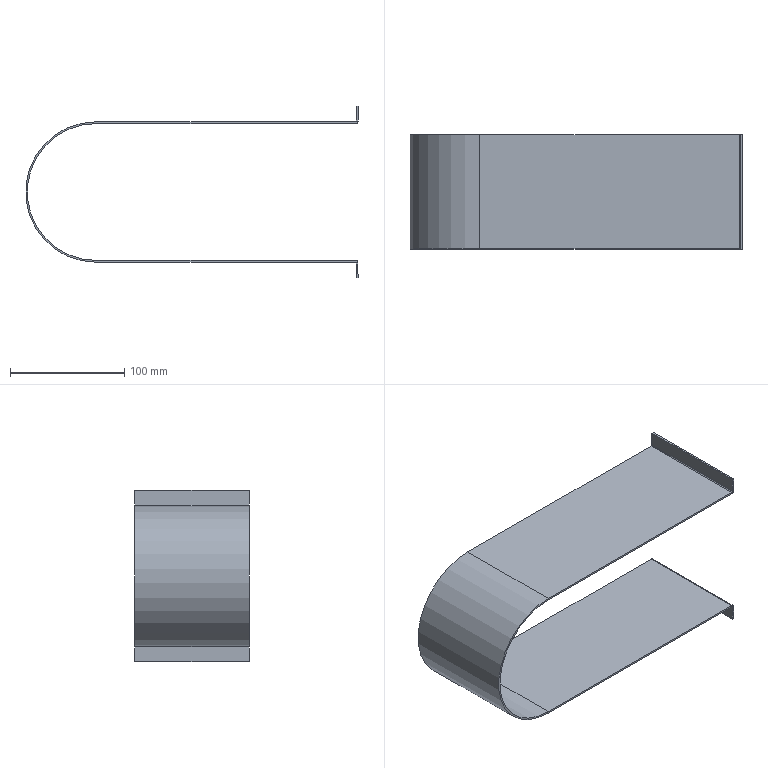Part | SolidWorks | features BaseBody 1 | 1 solid | 18 faces | box 291.5 x 100 x 150 mm | volume 101486 mm3 | plane 12 | cylinder 6 | commonest cylinder face diameters 1.473 x2 4.473 x2 120 x1 123 x1
STEP:
#1=CARTESIAN_POINT('',(-115.,100.,60.));
#2=VERTEX_POINT('',#1);
#3=CARTESIAN_POINT('',(112.763,100.,60.));
#4=VERTEX_POINT('',#3);
#5=CARTESIAN_POINT('',(-115.,100.,60.));
#6=DIRECTION('',(1.,0.,0.));
#7=VECTOR('',#6,1000.);
#8=LINE('',#5,#7);
#9=EDGE_CURVE('',#2,#4,#8,.T.);
#10=ORIENTED_EDGE('',*,*,#9,.T.);
#11=CARTESIAN_POINT('',(112.763,0.,60.));
#12=VERTEX_POINT('',#11);
#13=CARTESIAN_POINT('',(112.763,100.,60.));
#14=DIRECTION('',(0.,-1.,0.));
#15=VECTOR('',#14,1000.);
#16=LINE('',#13,#15);
#17=EDGE_CURVE('',#4,#12,#16,.T.);
#18=ORIENTED_EDGE('',*,*,#17,.T.);
#19=CARTESIAN_POINT('',(-115.,0.,60.));
#20=VERTEX_POINT('',#19);
#21=CARTESIAN_POINT('',(-115.,0.,60.));
#22=DIRECTION('',(-1.,0.,0.));
#23=VECTOR('',#22,1000.);
#24=LINE('',#21,#23);
#25=EDGE_CURVE('',#12,#20,#24,.T.);
#26=ORIENTED_EDGE('',*,*,#25,.T.);
#27=CARTESIAN_POINT('',(-115.,100.,60.));
#28=DIRECTION('',(0.,1.,0.));
#29=VECTOR('',#28,1000.);
#30=LINE('',#27,#29);
#31=EDGE_CURVE('',#20,#2,#30,.T.);
#32=ORIENTED_EDGE('',*,*,#31,.T.);
#33=EDGE_LOOP('',(#10,#18,#26,#32));
#34=FACE_OUTER_BOUND('',#33,.T.);
#35=CARTESIAN_POINT('',(-115.,100.,60.));
#36=DIRECTION('',(0.,0.,-1.));
#37=DIRECTION('',(-1.,0.,0.));
#38=AXIS2_PLACEMENT_3D('',#35,#36,#37);
#39=PLANE('',#38);
#40=ADVANCED_FACE('',(#34),#39,.T.);
#41=CARTESIAN_POINT('',(115.,100.,62.237));
#42=VERTEX_POINT('',#41);
#43=CARTESIAN_POINT('',(112.763,100.,62.237));
#44=DIRECTION('',(0.,-1.,0.));
#45=DIRECTION('',(0.,0.,-1.));
#46=AXIS2_PLACEMENT_3D('',#43,#44,#45);
#47=CIRCLE('',#46,2.237);
#48=EDGE_CURVE('',#4,#42,#47,.T.);
#49=ORIENTED_EDGE('',*,*,#48,.T.);
#50=CARTESIAN_POINT('',(115.,0.,62.237));
#51=VERTEX_POINT('',#50);
#52=CARTESIAN_POINT('',(115.,100.,62.237));
#53=DIRECTION('',(0.,-1.,0.));
#54=VECTOR('',#53,1000.);
#55=LINE('',#52,#54);
#56=EDGE_CURVE('',#42,#51,#55,.T.);
#57=ORIENTED_EDGE('',*,*,#56,.T.);
#58=CARTESIAN_POINT('',(112.763,0.,62.237));
#59=DIRECTION('',(0.,1.,0.));
#60=DIRECTION('',(0.,0.,-1.));
#61=AXIS2_PLACEMENT_3D('',#58,#59,#60);
#62=CIRCLE('',#61,2.237);
#63=EDGE_CURVE('',#51,#12,#62,.T.);
#64=ORIENTED_EDGE('',*,*,#63,.T.);
#65=ORIENTED_EDGE('',*,*,#17,.F.);
#66=EDGE_LOOP('',(#49,#57,#64,#65));
#67=FACE_OUTER_BOUND('',#66,.T.);
#68=CARTESIAN_POINT('',(112.763,100.,62.237));
#69=DIRECTION('',(0.,-1.,0.));
#70=DIRECTION('',(0.,0.,-1.));
#71=AXIS2_PLACEMENT_3D('',#68,#69,#70);
#72=CYLINDRICAL_SURFACE('',#71,2.237);
#73=ADVANCED_FACE('',(#67),#72,.T.);
#74=CARTESIAN_POINT('',(-115.,100.,61.5));
#75=VERTEX_POINT('',#74);
#76=CARTESIAN_POINT('',(112.763,100.,61.5));
#77=VERTEX_POINT('',#76);
#78=CARTESIAN_POINT('',(-115.,100.,61.5));
#79=DIRECTION('',(1.,0.,0.));
#80=VECTOR('',#79,1000.);
#81=LINE('',#78,#80);
#82=EDGE_CURVE('',#75,#77,#81,.T.);
#83=ORIENTED_EDGE('',*,*,#82,.T.);
#84=CARTESIAN_POINT('',(113.5,100.,62.237));
#85=VERTEX_POINT('',#84);
#86=CARTESIAN_POINT('',(112.763,100.,62.237));
#87=DIRECTION('',(0.,-1.,0.));
#88=DIRECTION('',(0.,0.,-1.));
#89=AXIS2_PLACEMENT_3D('',#86,#87,#88);
#90=CIRCLE('',#89,0.7366);
#91=EDGE_CURVE('',#77,#85,#90,.T.);
#92=ORIENTED_EDGE('',*,*,#91,.T.);
#93=CARTESIAN_POINT('',(113.5,100.,75.));
#94=VERTEX_POINT('',#93);
#95=CARTESIAN_POINT('',(113.5,100.,61.5));
#96=DIRECTION('',(0.,0.,1.));
#97=VECTOR('',#96,1000.);
#98=LINE('',#95,#97);
#99=EDGE_CURVE('',#85,#94,#98,.T.);
#100=ORIENTED_EDGE('',*,*,#99,.T.);
#101=CARTESIAN_POINT('',(115.,100.,75.));
#102=VERTEX_POINT('',#101);
#103=CARTESIAN_POINT('',(115.,100.,75.));
#104=DIRECTION('',(-1.,0.,0.));
#105=VECTOR('',#104,1000.);
#106=LINE('',#103,#105);
#107=EDGE_CURVE('',#102,#94,#106,.T.);
#108=ORIENTED_EDGE('',*,*,#107,.F.);
#109=CARTESIAN_POINT('',(115.,100.,60.));
#110=DIRECTION('',(0.,0.,1.));
#111=VECTOR('',#110,1000.);
#112=LINE('',#109,#111);
#113=EDGE_CURVE('',#42,#102,#112,.T.);
#114=ORIENTED_EDGE('',*,*,#113,.F.);
#115=ORIENTED_EDGE('',*,*,#48,.F.);
#116=ORIENTED_EDGE('',*,*,#9,.F.);
#117=CARTESIAN_POINT('',(-115.,100.,-60.));
#118=VERTEX_POINT('',#117);
#119=CARTESIAN_POINT('',(-115.,100.,0.));
#120=DIRECTION('',(0.,-1.,0.));
#121=DIRECTION('',(0.,0.,-1.));
#122=AXIS2_PLACEMENT_3D('',#119,#120,#121);
#123=CIRCLE('',#122,60.);
#124=EDGE_CURVE('',#2,#118,#123,.T.);
#125=ORIENTED_EDGE('',*,*,#124,.T.);
#126=CARTESIAN_POINT('',(112.763,100.,-60.));
#127=VERTEX_POINT('',#126);
#128=CARTESIAN_POINT('',(-115.,100.,-60.));
#129=DIRECTION('',(-1.,0.,0.));
#130=VECTOR('',#129,1000.);
#131=LINE('',#128,#130);
#132=EDGE_CURVE('',#127,#118,#131,.T.);
#133=ORIENTED_EDGE('',*,*,#132,.F.);
#134=CARTESIAN_POINT('',(115.,100.,-62.237));
#135=VERTEX_POINT('',#134);
#136=CARTESIAN_POINT('',(112.763,100.,-62.237));
#137=DIRECTION('',(0.,-1.,0.));
#138=DIRECTION('',(0.,0.,-1.));
#139=AXIS2_PLACEMENT_3D('',#136,#137,#138);
#140=CIRCLE('',#139,2.237);
#141=EDGE_CURVE('',#135,#127,#140,.T.);
#142=ORIENTED_EDGE('',*,*,#141,.F.);
#143=CARTESIAN_POINT('',(115.,100.,-75.));
#144=VERTEX_POINT('',#143);
#145=CARTESIAN_POINT('',(115.,100.,-60.));
#146=DIRECTION('',(0.,0.,1.));
#147=VECTOR('',#146,1000.);
#148=LINE('',#145,#147);
#149=EDGE_CURVE('',#144,#135,#148,.T.);
#150=ORIENTED_EDGE('',*,*,#149,.F.);
#151=CARTESIAN_POINT('',(113.5,100.,-75.));
#152=VERTEX_POINT('',#151);
#153=CARTESIAN_POINT('',(112.763,100.,-75.));
#154=DIRECTION('',(-1.,0.,0.));
#155=VECTOR('',#154,1000.);
#156=LINE('',#153,#155);
#157=EDGE_CURVE('',#144,#152,#156,.T.);
#158=ORIENTED_EDGE('',*,*,#157,.T.);
#159=CARTESIAN_POINT('',(113.5,100.,-62.237));
#160=VERTEX_POINT('',#159);
#161=CARTESIAN_POINT('',(113.5,100.,62.237));
#162=DIRECTION('',(0.,0.,1.));
#163=VECTOR('',#162,1000.);
#164=LINE('',#161,#163);
#165=EDGE_CURVE('',#152,#160,#164,.T.);
#166=ORIENTED_EDGE('',*,*,#165,.T.);
#167=CARTESIAN_POINT('',(112.763,100.,-61.5));
#168=VERTEX_POINT('',#167);
#169=CARTESIAN_POINT('',(112.763,100.,-62.237));
#170=DIRECTION('',(0.,-1.,0.));
#171=DIRECTION('',(0.,0.,-1.));
#172=AXIS2_PLACEMENT_3D('',#169,#170,#171);
#173=CIRCLE('',#172,0.7366);
#174=EDGE_CURVE('',#160,#168,#173,.T.);
#175=ORIENTED_EDGE('',*,*,#174,.T.);
#176=CARTESIAN_POINT('',(-115.,100.,-61.5));
#177=VERTEX_POINT('',#176);
#178=CARTESIAN_POINT('',(113.5,100.,-61.5));
#179=DIRECTION('',(-1.,0.,0.));
#180=VECTOR('',#179,1000.);
#181=LINE('',#178,#180);
#182=EDGE_CURVE('',#168,#177,#181,.T.);
#183=ORIENTED_EDGE('',*,*,#182,.T.);
#184=CARTESIAN_POINT('',(-115.,100.,0.));
#185=DIRECTION('',(0.,1.,0.));
#186=DIRECTION('',(0.,0.,-1.));
#187=AXIS2_PLACEMENT_3D('',#184,#185,#186);
#188=CIRCLE('',#187,61.5);
#189=EDGE_CURVE('',#177,#75,#188,.T.);
#190=ORIENTED_EDGE('',*,*,#189,.T.);
#191=EDGE_LOOP('',(#83,#92,#100,#108,#114,#115,#116,#125,#133,#142,#150,#158,#166,#175,#183,#190));
#192=FACE_OUTER_BOUND('',#191,.T.);
#193=CARTESIAN_POINT('',(-115.,100.,-61.5));
#194=DIRECTION('',(0.,1.,0.));
#195=DIRECTION('',(0.,0.,1.));
#196=AXIS2_PLACEMENT_3D('',#193,#194,#195);
#197=PLANE('',#196);
#198=ADVANCED_FACE('',(#192),#197,.T.);
#199=CARTESIAN_POINT('',(-115.,0.,-60.));
#200=VERTEX_POINT('',#199);
#201=CARTESIAN_POINT('',(-115.,100.,-60.));
#202=DIRECTION('',(0.,-1.,0.));
#203=VECTOR('',#202,1000.);
#204=LINE('',#201,#203);
#205=EDGE_CURVE('',#118,#200,#204,.T.);
#206=ORIENTED_EDGE('',*,*,#205,.F.);
#207=ORIENTED_EDGE('',*,*,#124,.F.);
#208=ORIENTED_EDGE('',*,*,#31,.F.);
#209=CARTESIAN_POINT('',(-115.,0.,0.));
#210=DIRECTION('',(0.,1.,0.));
#211=DIRECTION('',(0.,0.,-1.));
#212=AXIS2_PLACEMENT_3D('',#209,#210,#211);
#213=CIRCLE('',#212,60.);
#214=EDGE_CURVE('',#200,#20,#213,.T.);
#215=ORIENTED_EDGE('',*,*,#214,.F.);
#216=EDGE_LOOP('',(#206,#207,#208,#215));
#217=FACE_OUTER_BOUND('',#216,.T.);
#218=CARTESIAN_POINT('',(-115.,100.,0.));
#219=DIRECTION('',(0.,-1.,0.));
#220=DIRECTION('',(0.,0.,-1.));
#221=AXIS2_PLACEMENT_3D('',#218,#219,#220);
#222=CYLINDRICAL_SURFACE('',#221,60.);
#223=ADVANCED_FACE('',(#217),#222,.F.);
#224=CARTESIAN_POINT('',(112.763,0.,61.5));
#225=VERTEX_POINT('',#224);
#226=CARTESIAN_POINT('',(-115.,0.,61.5));
#227=VERTEX_POINT('',#226);
#228=CARTESIAN_POINT('',(113.5,0.,61.5));
#229=DIRECTION('',(-1.,0.,0.));
#230=VECTOR('',#229,1000.);
#231=LINE('',#228,#230);
#232=EDGE_CURVE('',#225,#227,#231,.T.);
#233=ORIENTED_EDGE('',*,*,#232,.T.);
#234=CARTESIAN_POINT('',(-115.,0.,-61.5));
#235=VERTEX_POINT('',#234);
#236=CARTESIAN_POINT('',(-115.,0.,0.));
#237=DIRECTION('',(0.,-1.,0.));
#238=DIRECTION('',(0.,0.,-1.));
#239=AXIS2_PLACEMENT_3D('',#236,#237,#238);
#240=CIRCLE('',#239,61.5);
#241=EDGE_CURVE('',#227,#235,#240,.T.);
#242=ORIENTED_EDGE('',*,*,#241,.T.);
#243=CARTESIAN_POINT('',(112.763,0.,-61.5));
#244=VERTEX_POINT('',#243);
#245=CARTESIAN_POINT('',(-115.,0.,-61.5));
#246=DIRECTION('',(1.,0.,0.));
#247=VECTOR('',#246,1000.);
#248=LINE('',#245,#247);
#249=EDGE_CURVE('',#235,#244,#248,.T.);
#250=ORIENTED_EDGE('',*,*,#249,.T.);
#251=CARTESIAN_POINT('',(113.5,0.,-62.237));
#252=VERTEX_POINT('',#251);
#253=CARTESIAN_POINT('',(112.763,0.,-62.237));
#254=DIRECTION('',(0.,1.,0.));
#255=DIRECTION('',(0.,0.,-1.));
#256=AXIS2_PLACEMENT_3D('',#253,#254,#255);
#257=CIRCLE('',#256,0.7366);
#258=EDGE_CURVE('',#244,#252,#257,.T.);
#259=ORIENTED_EDGE('',*,*,#258,.T.);
#260=CARTESIAN_POINT('',(113.5,0.,-75.));
#261=VERTEX_POINT('',#260);
#262=CARTESIAN_POINT('',(113.5,0.,-61.5));
#263=DIRECTION('',(0.,0.,-1.));
#264=VECTOR('',#263,1000.);
#265=LINE('',#262,#264);
#266=EDGE_CURVE('',#252,#261,#265,.T.);
#267=ORIENTED_EDGE('',*,*,#266,.T.);
#268=CARTESIAN_POINT('',(115.,0.,-75.));
#269=VERTEX_POINT('',#268);
#270=CARTESIAN_POINT('',(113.5,0.,-75.));
#271=DIRECTION('',(-1.,0.,0.));
#272=VECTOR('',#271,1000.);
#273=LINE('',#270,#272);
#274=EDGE_CURVE('',#269,#261,#273,.T.);
#275=ORIENTED_EDGE('',*,*,#274,.F.);
#276=CARTESIAN_POINT('',(115.,0.,-62.237));
#277=VERTEX_POINT('',#276);
#278=CARTESIAN_POINT('',(115.,0.,-60.));
#279=DIRECTION('',(0.,0.,-1.));
#280=VECTOR('',#279,1000.);
#281=LINE('',#278,#280);
#282=EDGE_CURVE('',#277,#269,#281,.T.);
#283=ORIENTED_EDGE('',*,*,#282,.F.);
#284=CARTESIAN_POINT('',(112.763,0.,-60.));
#285=VERTEX_POINT('',#284);
#286=CARTESIAN_POINT('',(112.763,0.,-62.237));
#287=DIRECTION('',(0.,1.,0.));
#288=DIRECTION('',(0.,0.,-1.));
#289=AXIS2_PLACEMENT_3D('',#286,#287,#288);
#290=CIRCLE('',#289,2.237);
#291=EDGE_CURVE('',#285,#277,#290,.T.);
#292=ORIENTED_EDGE('',*,*,#291,.F.);
#293=CARTESIAN_POINT('',(-115.,0.,-60.));
#294=DIRECTION('',(1.,0.,0.));
#295=VECTOR('',#294,1000.);
#296=LINE('',#293,#295);
#297=EDGE_CURVE('',#200,#285,#296,.T.);
#298=ORIENTED_EDGE('',*,*,#297,.F.);
#299=ORIENTED_EDGE('',*,*,#214,.T.);
#300=ORIENTED_EDGE('',*,*,#25,.F.);
#301=ORIENTED_EDGE('',*,*,#63,.F.);
#302=CARTESIAN_POINT('',(115.,0.,75.));
#303=VERTEX_POINT('',#302);
#304=CARTESIAN_POINT('',(115.,0.,60.));
#305=DIRECTION('',(0.,0.,-1.));
#306=VECTOR('',#305,1000.);
#307=LINE('',#304,#306);
#308=EDGE_CURVE('',#303,#51,#307,.T.);
#309=ORIENTED_EDGE('',*,*,#308,.F.);
#310=CARTESIAN_POINT('',(113.5,0.,75.));
#311=VERTEX_POINT('',#310);
#312=CARTESIAN_POINT('',(115.,0.,75.));
#313=DIRECTION('',(1.,0.,0.));
#314=VECTOR('',#313,1000.);
#315=LINE('',#312,#314);
#316=EDGE_CURVE('',#311,#303,#315,.T.);
#317=ORIENTED_EDGE('',*,*,#316,.F.);
#318=CARTESIAN_POINT('',(113.5,0.,62.237));
#319=VERTEX_POINT('',#318);
#320=CARTESIAN_POINT('',(113.5,0.,62.237));
#321=DIRECTION('',(0.,0.,1.));
#322=VECTOR('',#321,1000.);
#323=LINE('',#320,#322);
#324=EDGE_CURVE('',#319,#311,#323,.T.);
#325=ORIENTED_EDGE('',*,*,#324,.F.);
#326=CARTESIAN_POINT('',(112.763,0.,62.237));
#327=DIRECTION('',(0.,1.,0.));
#328=DIRECTION('',(0.,0.,-1.));
#329=AXIS2_PLACEMENT_3D('',#326,#327,#328);
#330=CIRCLE('',#329,0.7366);
#331=EDGE_CURVE('',#319,#225,#330,.T.);
#332=ORIENTED_EDGE('',*,*,#331,.T.);
#333=EDGE_LOOP('',(#233,#242,#250,#259,#267,#275,#283,#292,#298,#299,#300,#301,#309,#317,#325,#332));
#334=FACE_OUTER_BOUND('',#333,.T.);
#335=CARTESIAN_POINT('',(113.5,0.,62.237));
#336=DIRECTION('',(0.,-1.,0.));
#337=DIRECTION('',(0.,0.,-1.));
#338=AXIS2_PLACEMENT_3D('',#335,#336,#337);
#339=PLANE('',#338);
#340=ADVANCED_FACE('',(#334),#339,.T.);
#341=ORIENTED_EDGE('',*,*,#113,.T.);
#342=CARTESIAN_POINT('',(115.,100.,75.));
#343=DIRECTION('',(0.,-1.,0.));
#344=VECTOR('',#343,1000.);
#345=LINE('',#342,#344);
#346=EDGE_CURVE('',#102,#303,#345,.T.);
#347=ORIENTED_EDGE('',*,*,#346,.T.);
#348=ORIENTED_EDGE('',*,*,#308,.T.);
#349=ORIENTED_EDGE('',*,*,#56,.F.);
#350=EDGE_LOOP('',(#341,#347,#348,#349));
#351=FACE_OUTER_BOUND('',#350,.T.);
#352=CARTESIAN_POINT('',(115.,100.,60.));
#353=DIRECTION('',(1.,0.,0.));
#354=DIRECTION('',(0.,0.,-1.));
#355=AXIS2_PLACEMENT_3D('',#352,#353,#354);
#356=PLANE('',#355);
#357=ADVANCED_FACE('',(#351),#356,.T.);
#358=CARTESIAN_POINT('',(112.763,100.,61.5));
#359=DIRECTION('',(0.,-1.,0.));
#360=VECTOR('',#359,1000.);
#361=LINE('',#358,#360);
#362=EDGE_CURVE('',#77,#225,#361,.T.);
#363=ORIENTED_EDGE('',*,*,#362,.F.);
#364=ORIENTED_EDGE('',*,*,#82,.F.);
#365=CARTESIAN_POINT('',(-115.,100.,61.5));
#366=DIRECTION('',(0.,1.,0.));
#367=VECTOR('',#366,1000.);
#368=LINE('',#365,#367);
#369=EDGE_CURVE('',#227,#75,#368,.T.);
#370=ORIENTED_EDGE('',*,*,#369,.F.);
#371=ORIENTED_EDGE('',*,*,#232,.F.);
#372=EDGE_LOOP('',(#363,#364,#370,#371));
#373=FACE_OUTER_BOUND('',#372,.T.);
#374=CARTESIAN_POINT('',(-115.,100.,61.5));
#375=DIRECTION('',(0.,0.,-1.));
#376=DIRECTION('',(-1.,0.,0.));
#377=AXIS2_PLACEMENT_3D('',#374,#375,#376);
#378=PLANE('',#377);
#379=ADVANCED_FACE('',(#373),#378,.F.);
#380=ORIENTED_EDGE('',*,*,#132,.T.);
#381=ORIENTED_EDGE('',*,*,#205,.T.);
#382=ORIENTED_EDGE('',*,*,#297,.T.);
#383=CARTESIAN_POINT('',(112.763,100.,-60.));
#384=DIRECTION('',(0.,1.,0.));
#385=VECTOR('',#384,1000.);
#386=LINE('',#383,#385);
#387=EDGE_CURVE('',#285,#127,#386,.T.);
#388=ORIENTED_EDGE('',*,*,#387,.T.);
#389=EDGE_LOOP('',(#380,#381,#382,#388));
#390=FACE_OUTER_BOUND('',#389,.T.);
#391=CARTESIAN_POINT('',(-115.,100.,-60.));
#392=DIRECTION('',(0.,0.,1.));
#393=DIRECTION('',(1.,0.,0.));
#394=AXIS2_PLACEMENT_3D('',#391,#392,#393);
#395=PLANE('',#394);
#396=ADVANCED_FACE('',(#390),#395,.T.);
#397=ORIENTED_EDGE('',*,*,#107,.T.);
#398=CARTESIAN_POINT('',(113.5,100.,75.));
#399=DIRECTION('',(0.,-1.,0.));
#400=VECTOR('',#399,1000.);
#401=LINE('',#398,#400);
#402=EDGE_CURVE('',#94,#311,#401,.T.);
#403=ORIENTED_EDGE('',*,*,#402,.T.);
#404=ORIENTED_EDGE('',*,*,#316,.T.);
#405=ORIENTED_EDGE('',*,*,#346,.F.);
#406=EDGE_LOOP('',(#397,#403,#404,#405));
#407=FACE_OUTER_BOUND('',#406,.T.);
#408=CARTESIAN_POINT('',(115.,100.,75.));
#409=DIRECTION('',(0.,0.,1.));
#410=DIRECTION('',(1.,0.,0.));
#411=AXIS2_PLACEMENT_3D('',#408,#409,#410);
#412=PLANE('',#411);
#413=ADVANCED_FACE('',(#407),#412,.T.);
#414=CARTESIAN_POINT('',(113.5,100.,62.237));
#415=DIRECTION('',(0.,-1.,0.));
#416=VECTOR('',#415,1000.);
#417=LINE('',#414,#416);
#418=EDGE_CURVE('',#85,#319,#417,.T.);
#419=ORIENTED_EDGE('',*,*,#418,.F.);
#420=ORIENTED_EDGE('',*,*,#91,.F.);
#421=ORIENTED_EDGE('',*,*,#362,.T.);
#422=ORIENTED_EDGE('',*,*,#331,.F.);
#423=EDGE_LOOP('',(#419,#420,#421,#422));
#424=FACE_OUTER_BOUND('',#423,.T.);
#425=CARTESIAN_POINT('',(112.763,100.,62.237));
#426=DIRECTION('',(0.,-1.,0.));
#427=DIRECTION('',(0.,0.,-1.));
#428=AXIS2_PLACEMENT_3D('',#425,#426,#427);
#429=CYLINDRICAL_SURFACE('',#428,0.7366);
#430=ADVANCED_FACE('',(#424),#429,.F.);
#431=ORIENTED_EDGE('',*,*,#189,.F.);
#432=CARTESIAN_POINT('',(-115.,100.,-61.5));
#433=DIRECTION('',(0.,-1.,0.));
#434=VECTOR('',#433,1000.);
#435=LINE('',#432,#434);
#436=EDGE_CURVE('',#177,#235,#435,.T.);
#437=ORIENTED_EDGE('',*,*,#436,.T.);
#438=ORIENTED_EDGE('',*,*,#241,.F.);
#439=ORIENTED_EDGE('',*,*,#369,.T.);
#440=EDGE_LOOP('',(#431,#437,#438,#439));
#441=FACE_OUTER_BOUND('',#440,.T.);
#442=CARTESIAN_POINT('',(-115.,100.,0.));
#443=DIRECTION('',(0.,-1.,0.));
#444=DIRECTION('',(0.,0.,-1.));
#445=AXIS2_PLACEMENT_3D('',#442,#443,#444);
#446=CYLINDRICAL_SURFACE('',#445,61.5);
#447=ADVANCED_FACE('',(#441),#446,.T.);
#448=ORIENTED_EDGE('',*,*,#141,.T.);
#449=ORIENTED_EDGE('',*,*,#387,.F.);
#450=ORIENTED_EDGE('',*,*,#291,.T.);
#451=CARTESIAN_POINT('',(115.,100.,-62.237));
#452=DIRECTION('',(0.,1.,0.));
#453=VECTOR('',#452,1000.);
#454=LINE('',#451,#453);
#455=EDGE_CURVE('',#277,#135,#454,.T.);
#456=ORIENTED_EDGE('',*,*,#455,.T.);
#457=EDGE_LOOP('',(#448,#449,#450,#456));
#458=FACE_OUTER_BOUND('',#457,.T.);
#459=CARTESIAN_POINT('',(112.763,100.,-62.237));
#460=DIRECTION('',(0.,-1.,0.));
#461=DIRECTION('',(0.,0.,-1.));
#462=AXIS2_PLACEMENT_3D('',#459,#460,#461);
#463=CYLINDRICAL_SURFACE('',#462,2.237);
#464=ADVANCED_FACE('',(#458),#463,.T.);
#465=ORIENTED_EDGE('',*,*,#402,.F.);
#466=ORIENTED_EDGE('',*,*,#99,.F.);
#467=ORIENTED_EDGE('',*,*,#418,.T.);
#468=ORIENTED_EDGE('',*,*,#324,.T.);
#469=EDGE_LOOP('',(#465,#466,#467,#468));
#470=FACE_OUTER_BOUND('',#469,.T.);
#471=CARTESIAN_POINT('',(113.5,100.,60.));
#472=DIRECTION('',(1.,0.,0.));
#473=DIRECTION('',(0.,0.,-1.));
#474=AXIS2_PLACEMENT_3D('',#471,#472,#473);
#475=PLANE('',#474);
#476=ADVANCED_FACE('',(#470),#475,.F.);
#477=ORIENTED_EDGE('',*,*,#436,.F.);
#478=ORIENTED_EDGE('',*,*,#182,.F.);
#479=CARTESIAN_POINT('',(112.763,100.,-61.5));
#480=DIRECTION('',(0.,1.,0.));
#481=VECTOR('',#480,1000.);
#482=LINE('',#479,#481);
#483=EDGE_CURVE('',#244,#168,#482,.T.);
#484=ORIENTED_EDGE('',*,*,#483,.F.);
#485=ORIENTED_EDGE('',*,*,#249,.F.);
#486=EDGE_LOOP('',(#477,#478,#484,#485));
#487=FACE_OUTER_BOUND('',#486,.T.);
#488=CARTESIAN_POINT('',(-115.,100.,-61.5));
#489=DIRECTION('',(0.,0.,1.));
#490=DIRECTION('',(1.,0.,0.));
#491=AXIS2_PLACEMENT_3D('',#488,#489,#490);
#492=PLANE('',#491);
#493=ADVANCED_FACE('',(#487),#492,.F.);
#494=ORIENTED_EDGE('',*,*,#149,.T.);
#495=ORIENTED_EDGE('',*,*,#455,.F.);
#496=ORIENTED_EDGE('',*,*,#282,.T.);
#497=CARTESIAN_POINT('',(115.,100.,-75.));
#498=DIRECTION('',(0.,1.,0.));
#499=VECTOR('',#498,1000.);
#500=LINE('',#497,#499);
#501=EDGE_CURVE('',#269,#144,#500,.T.);
#502=ORIENTED_EDGE('',*,*,#501,.T.);
#503=EDGE_LOOP('',(#494,#495,#496,#502));
#504=FACE_OUTER_BOUND('',#503,.T.);
#505=CARTESIAN_POINT('',(115.,100.,-60.));
#506=DIRECTION('',(1.,0.,0.));
#507=DIRECTION('',(0.,0.,-1.));
#508=AXIS2_PLACEMENT_3D('',#505,#506,#507);
#509=PLANE('',#508);
#510=ADVANCED_FACE('',(#504),#509,.T.);
#511=ORIENTED_EDGE('',*,*,#483,.T.);
#512=ORIENTED_EDGE('',*,*,#174,.F.);
#513=CARTESIAN_POINT('',(113.5,100.,-62.237));
#514=DIRECTION('',(0.,1.,0.));
#515=VECTOR('',#514,1000.);
#516=LINE('',#513,#515);
#517=EDGE_CURVE('',#252,#160,#516,.T.);
#518=ORIENTED_EDGE('',*,*,#517,.F.);
#519=ORIENTED_EDGE('',*,*,#258,.F.);
#520=EDGE_LOOP('',(#511,#512,#518,#519));
#521=FACE_OUTER_BOUND('',#520,.T.);
#522=CARTESIAN_POINT('',(112.763,100.,-62.237));
#523=DIRECTION('',(0.,-1.,0.));
#524=DIRECTION('',(0.,0.,-1.));
#525=AXIS2_PLACEMENT_3D('',#522,#523,#524);
#526=CYLINDRICAL_SURFACE('',#525,0.7366);
#527=ADVANCED_FACE('',(#521),#526,.F.);
#528=ORIENTED_EDGE('',*,*,#157,.F.);
#529=ORIENTED_EDGE('',*,*,#501,.F.);
#530=ORIENTED_EDGE('',*,*,#274,.T.);
#531=CARTESIAN_POINT('',(113.5,100.,-75.));
#532=DIRECTION('',(0.,1.,0.));
#533=VECTOR('',#532,1000.);
#534=LINE('',#531,#533);
#535=EDGE_CURVE('',#261,#152,#534,.T.);
#536=ORIENTED_EDGE('',*,*,#535,.T.);
#537=EDGE_LOOP('',(#528,#529,#530,#536));
#538=FACE_OUTER_BOUND('',#537,.T.);
#539=CARTESIAN_POINT('',(113.5,100.,-75.));
#540=DIRECTION('',(0.,0.,-1.));
#541=DIRECTION('',(-1.,0.,0.));
#542=AXIS2_PLACEMENT_3D('',#539,#540,#541);
#543=PLANE('',#542);
#544=ADVANCED_FACE('',(#538),#543,.T.);
#545=ORIENTED_EDGE('',*,*,#517,.T.);
#546=ORIENTED_EDGE('',*,*,#165,.F.);
#547=ORIENTED_EDGE('',*,*,#535,.F.);
#548=ORIENTED_EDGE('',*,*,#266,.F.);
#549=EDGE_LOOP('',(#545,#546,#547,#548));
#550=FACE_OUTER_BOUND('',#549,.T.);
#551=CARTESIAN_POINT('',(113.5,100.,-60.));
#552=DIRECTION('',(1.,0.,0.));
#553=DIRECTION('',(0.,0.,-1.));
#554=AXIS2_PLACEMENT_3D('',#551,#552,#553);
#555=PLANE('',#554);
#556=ADVANCED_FACE('',(#550),#555,.F.);
#557=CLOSED_SHELL('',(#40,#73,#198,#223,#340,#357,#379,#396,#413,#430,#447,#464,#476,#493,#510,#527,#544,#556));
#558=MANIFOLD_SOLID_BREP('',#557);
#559=CARTESIAN_POINT('',(0.,0.,0.));
#560=DIRECTION('',(0.,0.,1.));
#561=DIRECTION('',(1.,0.,0.));
#562=AXIS2_PLACEMENT_3D('',#559,#560,#561);
#563=(LENGTH_UNIT()NAMED_UNIT(*)SI_UNIT(.MILLI.,.METRE.));
#564=UNCERTAINTY_MEASURE_WITH_UNIT(LENGTH_MEASURE(0.00001),#563,'','');
#565=(NAMED_UNIT(*)PLANE_ANGLE_UNIT()SI_UNIT($,.RADIAN.));
#566=(NAMED_UNIT(*)SI_UNIT($,.STERADIAN.)SOLID_ANGLE_UNIT());
#567=(GEOMETRIC_REPRESENTATION_CONTEXT(3)GLOBAL_UNCERTAINTY_ASSIGNED_CONTEXT((#564))GLOBAL_UNIT_ASSIGNED_CONTEXT((#563,#565,#566))REPRESENTATION_CONTEXT('',''));
#568=ADVANCED_BREP_SHAPE_REPRESENTATION('',(#558,#562),#567);